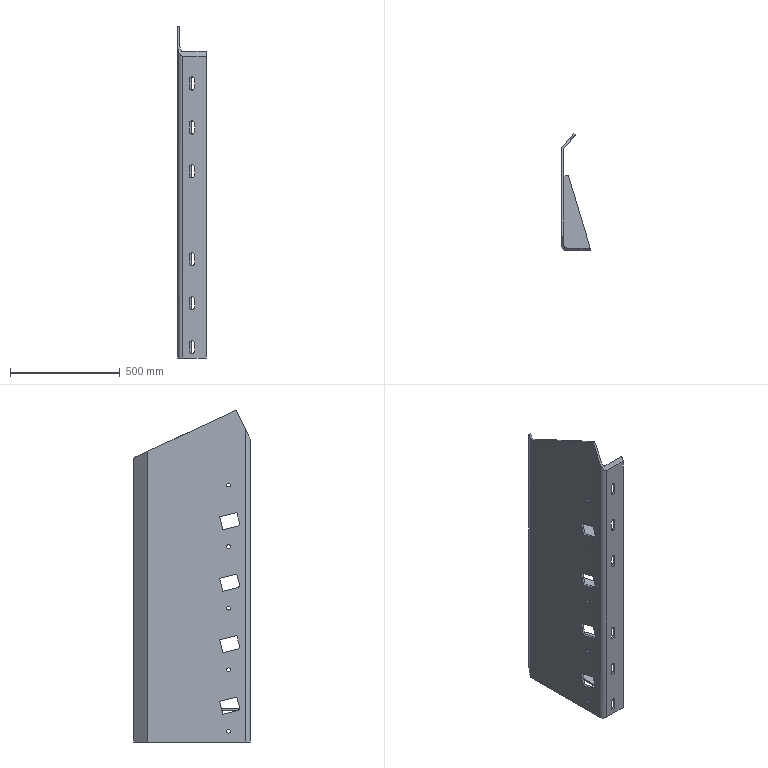Part | STEP file | Edge plate 8_Default<As machined> | 6 solids | 102 faces | box 130 x 532.359 x 1511 mm | volume 9898489 mm3 | plane 69 | cylinder 33 | commonest cylinder face diameters 24 x18 17 x10 30 x4 44 x1